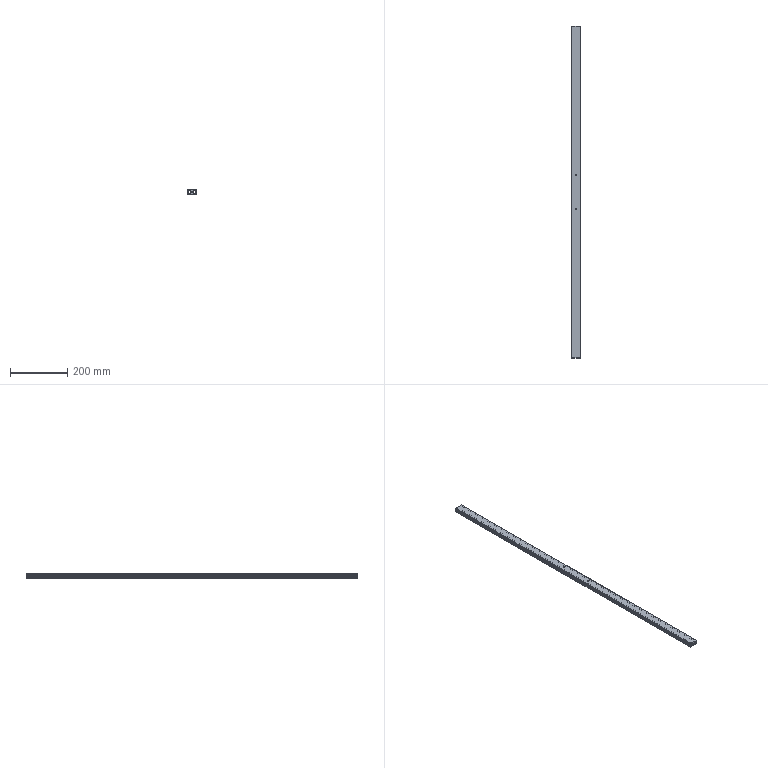Part | STEP file | GB1530T-6-30x15x1155-BASHOU | 1 solid | 60 faces | box 30 x 1157 x 15 mm | volume 281206 mm3 | cylinder 38 | plane 22 | commonest cylinder face diameters 2 x28 5 x8 5.2 x2